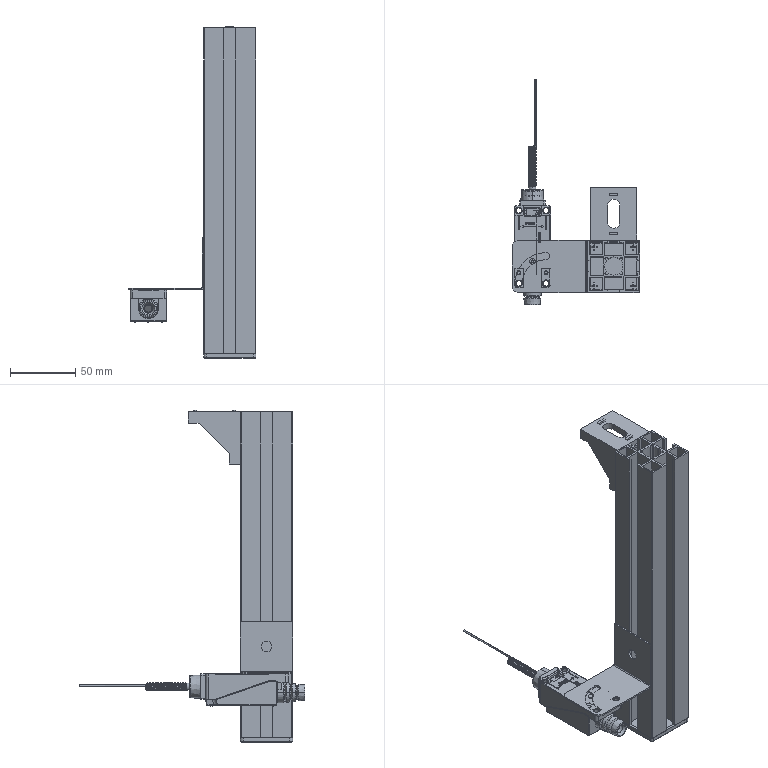Part | 4 solids | 1207 faces | box 98 x 173.5 x 255 mm | volume 154769 mm3 | plane 553 | cylinder 270 | spline 162 | cone 119 | torus 89 | sphere 14 | commonest cylinder face diameters 1 x53 3 x18 0.6 x16 1.5 x16 2.5 x16 1.56 x12